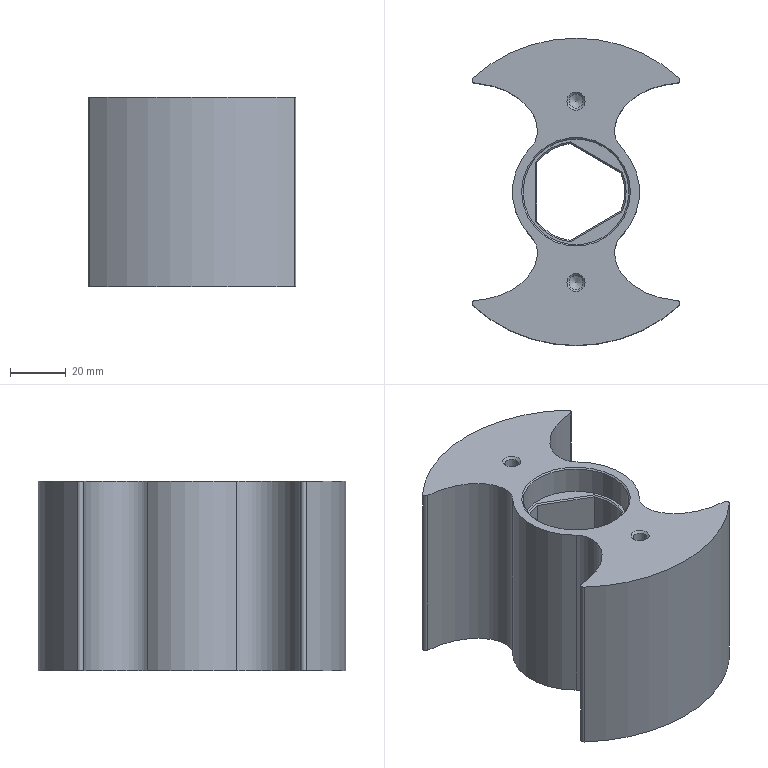NC program | NX | posted with a generic post | part box 74.46 x 110.159 x 68 mm
Lines 1 to 924 of 14265:
N10 G17 G21 G94 G90
(ZLEVEL_PROFILE_COPY_2 , TOOL : D25R0.5)
N12 T05 M6
N14 G54
N16 G17 G0 G90 X-62.643 Y50.68 S2000 M3
N18 G43 Z30. H5
N20 Z-0.349
N22 G94 G1 X-58.542 Y49.805 F1000.
N24 G3 X-56.163 Y50.576 R2.5
N26 G2 X-45.476 Y57.048 R21.659 F2200.
N28 X-34.718 Y57.049 R21.673
N30 G1 X-34.038 Y56.851
N32 G2 X-18.67 Y39.036 R21.585
N34 G1 X-18.667 Y39.034
N36 X-17.856 Y39.412
N38 X-17.06 Y39.763
N40 G2 X17.498 Y39.586 R43.327
N42 G1 X18.67 Y39.033
N44 G2 X19.13 Y41.403 R23.414
N46 G1 X19.344 Y42.145
N48 G2 X34.465 Y56.981 R21.564
N50 G1 X34.731 Y57.052
N52 G2 X45.481 Y57.045 R21.673
N54 X56.163 Y50.576 R21.656
N56 G3 X58.542 Y49.805 R2.5
N58 G1 X62.645 Y50.68
N60 G0 Z30.
N62 X-62.649 Y50.677
N64 Z-0.697
N66 G1 X-58.541 Y49.803 F1000.
N68 G3 X-56.163 Y50.576 R2.5
N70 G2 X-18.668 Y39.036 R21.625 F2200.
N72 X18.549 Y39.093 R43.271
N74 G1 X18.668 Y39.034
N76 G2 X56.163 Y50.576 R21.625
N78 G3 X58.541 Y49.803 R2.5
N80 G1 X62.649 Y50.677
N82 G0 Z30.
N84 X-62.649
N86 Z-1.046
N88 G1 X-58.541 Y49.803 F1000.
N90 G3 X-56.163 Y50.576 R2.5
N92 G2 X-18.668 Y39.036 R21.625 F2200.
N94 X18.549 Y39.093 R43.271
N96 G1 X18.668 Y39.034
N98 G2 X56.163 Y50.576 R21.625
N100 G3 X58.541 Y49.803 R2.5
N102 G1 X62.649 Y50.677
N104 G0 Z30.
N106 X-62.649
N108 Z-1.395
N110 G1 X-58.541 Y49.803 F1000.
N112 G3 X-56.163 Y50.576 R2.5
N114 G2 X-18.668 Y39.036 R21.625 F2200.
N116 X18.549 Y39.093 R43.271
N118 G1 X18.668 Y39.034
N120 G2 X56.163 Y50.576 R21.625
N122 G3 X58.541 Y49.803 R2.5
N124 G1 X62.649 Y50.677
N126 G0 Z30.
N128 X-62.649
N130 Z-1.744
N132 G1 X-58.541 Y49.803 F1000.
N134 G3 X-56.163 Y50.576 R2.5
N136 G2 X-18.668 Y39.036 R21.625 F2200.
N138 X18.549 Y39.093 R43.271
N140 G1 X18.668 Y39.034
N142 G2 X56.163 Y50.576 R21.625
N144 G3 X58.541 Y49.803 R2.5
N146 G1 X62.649 Y50.677
N148 G0 Z30.
N150 X-62.649
N152 Z-2.092
N154 G1 X-58.541 Y49.803 F1000.
N156 G3 X-56.163 Y50.576 R2.5
N158 G2 X-18.668 Y39.036 R21.625 F2200.
N160 X18.549 Y39.093 R43.271
N162 G1 X18.668 Y39.034
N164 G2 X56.163 Y50.576 R21.625
N166 G3 X58.541 Y49.803 R2.5
N168 G1 X62.649 Y50.677
N170 G0 Z30.
N172 X-62.649
N174 Z-2.441
N176 G1 X-58.541 Y49.803 F1000.
N178 G3 X-56.163 Y50.576 R2.5
N180 G2 X-18.668 Y39.036 R21.625 F2200.
N182 X18.549 Y39.093 R43.271
N184 G1 X18.668 Y39.034
N186 G2 X56.163 Y50.576 R21.625
N188 G3 X58.541 Y49.803 R2.5
N190 G1 X62.649 Y50.677
N192 G0 Z30.
N194 X-62.649
N196 Z-2.79
N198 G1 X-58.541 Y49.803 F1000.
N200 G3 X-56.163 Y50.576 R2.5
N202 G2 X-18.668 Y39.036 R21.625 F2200.
N204 X18.549 Y39.093 R43.271
N206 G1 X18.668 Y39.034
N208 G2 X56.163 Y50.576 R21.625
N210 G3 X58.541 Y49.803 R2.5
N212 G1 X62.649 Y50.677
N214 G0 Z30.
N216 X-62.649
N218 Z-3.138
N220 G1 X-58.541 Y49.803 F1000.
N222 G3 X-56.163 Y50.576 R2.5
N224 G2 X-18.668 Y39.036 R21.625 F2200.
N226 X18.549 Y39.093 R43.271
N228 G1 X18.668 Y39.034
N230 G2 X56.163 Y50.576 R21.625
N232 G3 X58.541 Y49.803 R2.5
N234 G1 X62.649 Y50.677
N236 G0 Z30.
N238 X-62.649
N240 Z-3.487
N242 G1 X-58.541 Y49.803 F1000.
N244 G3 X-56.163 Y50.576 R2.5
N246 G2 X-18.668 Y39.036 R21.625 F2200.
N248 X18.549 Y39.093 R43.271
N250 G1 X18.668 Y39.034
N252 G2 X56.163 Y50.576 R21.625
N254 G3 X58.541 Y49.803 R2.5
N256 G1 X62.649 Y50.677
N258 G0 Z30.
N260 X-62.649
N262 Z-3.836
N264 G1 X-58.541 Y49.803 F1000.
N266 G3 X-56.163 Y50.576 R2.5
N268 G2 X-18.668 Y39.036 R21.625 F2200.
N270 X18.549 Y39.093 R43.271
N272 G1 X18.668 Y39.034
N274 G2 X56.163 Y50.576 R21.625
N276 G3 X58.541 Y49.803 R2.5
N278 G1 X62.649 Y50.677
N280 G0 Z30.
N282 X-62.649
N284 Z-4.185
N286 G1 X-58.541 Y49.803 F1000.
N288 G3 X-56.163 Y50.576 R2.5
N290 G2 X-18.668 Y39.036 R21.625 F2200.
N292 X18.549 Y39.093 R43.271
N294 G1 X18.668 Y39.034
N296 G2 X56.163 Y50.576 R21.625
N298 G3 X58.541 Y49.803 R2.5
N300 G1 X62.649 Y50.677
N302 G0 Z30.
N304 X-62.649
N306 Z-4.533
N308 G1 X-58.541 Y49.803 F1000.
N310 G3 X-56.163 Y50.576 R2.5
N312 G2 X-18.668 Y39.036 R21.625 F2200.
N314 X18.549 Y39.093 R43.271
N316 G1 X18.668 Y39.034
N318 G2 X56.163 Y50.576 R21.625
N320 G3 X58.541 Y49.803 R2.5
N322 G1 X62.649 Y50.677
N324 G0 Z30.
N326 X-62.649
N328 Z-4.882
N330 G1 X-58.541 Y49.803 F1000.
N332 G3 X-56.163 Y50.576 R2.5
N334 G2 X-18.668 Y39.036 R21.625 F2200.
N336 X18.549 Y39.093 R43.271
N338 G1 X18.668 Y39.034
N340 G2 X56.163 Y50.576 R21.625
N342 G3 X58.541 Y49.803 R2.5
N344 G1 X62.649 Y50.677
N346 G0 Z30.
N348 X-62.649
N350 Z-5.231
N352 G1 X-58.541 Y49.803 F1000.
N354 G3 X-56.163 Y50.576 R2.5
N356 G2 X-18.668 Y39.036 R21.625 F2200.
N358 X18.549 Y39.093 R43.271
N360 G1 X18.668 Y39.034
N362 G2 X56.163 Y50.576 R21.625
N364 G3 X58.541 Y49.803 R2.5
N366 G1 X62.649 Y50.677
N368 G0 Z30.
N370 X-62.649
N372 Z-5.579
N374 G1 X-58.541 Y49.803 F1000.
N376 G3 X-56.163 Y50.576 R2.5
N378 G2 X-18.668 Y39.036 R21.625 F2200.
N380 X18.549 Y39.093 R43.271
N382 G1 X18.668 Y39.034
N384 G2 X56.163 Y50.576 R21.625
N386 G3 X58.541 Y49.803 R2.5
N388 G1 X62.649 Y50.677
N390 G0 Z30.
N392 X-62.649
N394 Z-5.928
N396 G1 X-58.541 Y49.803 F1000.
N398 G3 X-56.163 Y50.576 R2.5
N400 G2 X-18.668 Y39.036 R21.625 F2200.
N402 X18.549 Y39.093 R43.271
N404 G1 X18.668 Y39.035
N406 G2 X56.163 Y50.576 R21.625
N408 G3 X58.541 Y49.803 R2.5
N410 G1 X62.649 Y50.677
N412 G0 Z30.
N414 X-62.649
N416 Z-6.277
N418 G1 X-58.541 Y49.803 F1000.
N420 G3 X-56.163 Y50.576 R2.5
N422 G2 X-18.668 Y39.036 R21.625 F2200.
N424 X18.549 Y39.093 R43.271
N426 G1 X18.668 Y39.035
N428 G2 X56.163 Y50.576 R21.625
N430 G3 X58.541 Y49.803 R2.5
N432 G1 X62.649 Y50.677
N434 G0 Z30.
N436 X-62.649
N438 Z-6.626
N440 G1 X-58.541 Y49.803 F1000.
N442 G3 X-56.163 Y50.576 R2.5
N444 G2 X-18.668 Y39.036 R21.625 F2200.
N446 X18.549 Y39.093 R43.271
N448 G1 X18.668 Y39.035
N450 G2 X56.163 Y50.576 R21.625
N452 G3 X58.541 Y49.803 R2.5
N454 G1 X62.649 Y50.677
N456 G0 Z30.
N458 X-62.649
N460 Z-6.974
N462 G1 X-58.541 Y49.803 F1000.
N464 G3 X-56.163 Y50.576 R2.5
N466 G2 X-18.668 Y39.036 R21.625 F2200.
N468 X18.549 Y39.093 R43.271
N470 G1 X18.668 Y39.035
N472 G2 X56.163 Y50.576 R21.625
N474 G3 X58.541 Y49.803 R2.5
N476 G1 X62.649 Y50.677
N478 G0 Z30.
N480 X-62.649
N482 Z-7.323
N484 G1 X-58.541 Y49.803 F1000.
N486 G3 X-56.163 Y50.576 R2.5
N488 G2 X-18.668 Y39.036 R21.625 F2200.
N490 X18.549 Y39.093 R43.271
N492 G1 X18.668 Y39.035
N494 G2 X56.163 Y50.576 R21.625
N496 G3 X58.541 Y49.803 R2.5
N498 G1 X62.649 Y50.677
N500 G0 Z30.
N502 X-62.649
N504 Z-7.672
N506 G1 X-58.541 Y49.803 F1000.
N508 G3 X-56.163 Y50.576 R2.5
N510 G2 X-18.668 Y39.036 R21.625 F2200.
N512 X18.549 Y39.093 R43.271
N514 G1 X18.668 Y39.035
N516 G2 X56.163 Y50.576 R21.625
N518 G3 X58.541 Y49.803 R2.5
N520 G1 X62.649 Y50.677
N522 G0 Z30.
N524 X-62.649
N526 Z-8.021
N528 G1 X-58.541 Y49.803 F1000.
N530 G3 X-56.163 Y50.576 R2.5
N532 G2 X-18.668 Y39.036 R21.625 F2200.
N534 X18.549 Y39.093 R43.271
N536 G1 X18.668 Y39.035
N538 G2 X56.163 Y50.576 R21.625
N540 G3 X58.541 Y49.803 R2.5
N542 G1 X62.649 Y50.677
N544 G0 Z30.
N546 X-62.649
N548 Z-8.369
N550 G1 X-58.541 Y49.803 F1000.
N552 G3 X-56.163 Y50.576 R2.5
N554 G2 X-18.668 Y39.036 R21.625 F2200.
N556 X18.549 Y39.093 R43.271
N558 G1 X18.668 Y39.035
N560 G2 X56.163 Y50.576 R21.625
N562 G3 X58.541 Y49.803 R2.5
N564 G1 X62.649 Y50.677
N566 G0 Z30.
N568 X-62.649
N570 Z-8.718
N572 G1 X-58.541 Y49.803 F1000.
N574 G3 X-56.163 Y50.576 R2.5
N576 G2 X-18.668 Y39.036 R21.625 F2200.
N578 X18.549 Y39.093 R43.271
N580 G1 X18.668 Y39.035
N582 G2 X56.163 Y50.576 R21.625
N584 G3 X58.541 Y49.803 R2.5
N586 G1 X62.649 Y50.677
N588 G0 Z30.
N590 X-62.649
N592 Z-9.067
N594 G1 X-58.541 Y49.803 F1000.
N596 G3 X-56.163 Y50.576 R2.5
N598 G2 X-18.668 Y39.036 R21.625 F2200.
N600 X18.549 Y39.093 R43.271
N602 G1 X18.668 Y39.035
N604 G2 X56.163 Y50.576 R21.625
N606 G3 X58.541 Y49.803 R2.5
N608 G1 X62.649 Y50.677
N610 G0 Z30.
N612 X-62.649
N614 Z-9.415
N616 G1 X-58.541 Y49.803 F1000.
N618 G3 X-56.163 Y50.576 R2.5
N620 G2 X-18.668 Y39.036 R21.625 F2200.
N622 X18.549 Y39.093 R43.271
N624 G1 X18.668 Y39.035
N626 G2 X56.163 Y50.576 R21.625
N628 G3 X58.541 Y49.803 R2.5
N630 G1 X62.649 Y50.677
N632 G0 Z30.
N634 X-62.649
N636 Z-9.764
N638 G1 X-58.541 Y49.803 F1000.
N640 G3 X-56.163 Y50.576 R2.5
N642 G2 X-18.668 Y39.036 R21.625 F2200.
N644 X18.549 Y39.093 R43.271
N646 G1 X18.668 Y39.035
N648 G2 X56.163 Y50.576 R21.625
N650 G3 X58.541 Y49.803 R2.5
N652 G1 X62.649 Y50.677
N654 G0 Z30.
N656 X-62.649
N658 Z-10.113
N660 G1 X-58.541 Y49.803 F1000.
N662 G3 X-56.163 Y50.576 R2.5
N664 G2 X-18.668 Y39.036 R21.625 F2200.
N666 X18.549 Y39.093 R43.271
N668 G1 X18.668 Y39.035
N670 G2 X56.163 Y50.576 R21.625
N672 G3 X58.541 Y49.803 R2.5
N674 G1 X62.649 Y50.677
N676 G0 Z30.
N678 X-62.649
N680 Z-10.462
N682 G1 X-58.541 Y49.803 F1000.
N684 G3 X-56.163 Y50.576 R2.5
N686 G2 X-18.668 Y39.036 R21.625 F2200.
N688 X18.549 Y39.093 R43.271
N690 G1 X18.668 Y39.035
N692 G2 X56.163 Y50.576 R21.625
N694 G3 X58.541 Y49.803 R2.5
N696 G1 X62.649 Y50.677
N698 G0 Z30.
N700 X-62.649
N702 Z-10.81
N704 G1 X-58.541 Y49.803 F1000.
N706 G3 X-56.163 Y50.576 R2.5
N708 G2 X-18.668 Y39.036 R21.625 F2200.
N710 X18.549 Y39.093 R43.271
N712 G1 X18.668 Y39.035
N714 G2 X56.163 Y50.576 R21.625
N716 G3 X58.541 Y49.803 R2.5
N718 G1 X62.649 Y50.677
N720 G0 Z30.
N722 X-62.649
N724 Z-11.159
N726 G1 X-58.541 Y49.803 F1000.
N728 G3 X-56.163 Y50.576 R2.5
N730 G2 X-18.668 Y39.036 R21.625 F2200.
N732 X18.549 Y39.093 R43.271
N734 G1 X18.668 Y39.035
N736 G2 X56.163 Y50.576 R21.625
N738 G3 X58.541 Y49.803 R2.5
N740 G1 X62.649 Y50.677
N742 G0 Z30.
N744 X-62.649
N746 Z-11.508
N748 G1 X-58.541 Y49.803 F1000.
N750 G3 X-56.163 Y50.576 R2.5
N752 G2 X-18.668 Y39.036 R21.625 F2200.
N754 X18.549 Y39.093 R43.271
N756 G1 X18.668 Y39.035
N758 G2 X56.163 Y50.576 R21.625
N760 G3 X58.541 Y49.803 R2.5
N762 G1 X62.649 Y50.677
N764 G0 Z30.
N766 X-62.649
N768 Z-11.856
N770 G1 X-58.541 Y49.803 F1000.
N772 G3 X-56.163 Y50.576 R2.5
N774 G2 X-18.668 Y39.036 R21.625 F2200.
N776 X18.549 Y39.093 R43.271
N778 G1 X18.668 Y39.035
N780 G2 X56.163 Y50.576 R21.625
N782 G3 X58.541 Y49.803 R2.5
N784 G1 X62.649 Y50.677
N786 G0 Z30.
N788 X-62.649
N790 Z-12.205
N792 G1 X-58.541 Y49.803 F1000.
N794 G3 X-56.163 Y50.576 R2.5
N796 G2 X-18.668 Y39.036 R21.625 F2200.
N798 X18.549 Y39.093 R43.271
N800 G1 X18.668 Y39.035
N802 G2 X56.163 Y50.576 R21.625
N804 G3 X58.541 Y49.803 R2.5
N806 G1 X62.649 Y50.677
N808 G0 Z30.
N810 X-62.649
N812 Z-12.554
N814 G1 X-58.541 Y49.803 F1000.
N816 G3 X-56.163 Y50.576 R2.5
N818 G2 X-18.668 Y39.036 R21.625 F2200.
N820 X18.549 Y39.093 R43.271
N822 G1 X18.668 Y39.035
N824 G2 X56.163 Y50.576 R21.625
N826 G3 X58.541 Y49.803 R2.5
N828 G1 X62.649 Y50.677
N830 G0 Z30.
N832 X-62.649
N834 Z-12.903
N836 G1 X-58.541 Y49.803 F1000.
N838 G3 X-56.163 Y50.576 R2.5
N840 G2 X-18.668 Y39.036 R21.625 F2200.
N842 X18.549 Y39.093 R43.271
N844 G1 X18.668 Y39.035
N846 G2 X56.163 Y50.576 R21.625
N848 G3 X58.541 Y49.803 R2.5
N850 G1 X62.649 Y50.677
N852 G0 Z30.
N854 X-62.649
N856 Z-13.251
N858 G1 X-58.541 Y49.803 F1000.
N860 G3 X-56.163 Y50.576 R2.5
N862 G2 X-18.668 Y39.036 R21.625 F2200.
N864 X18.549 Y39.093 R43.271
N866 G1 X18.668 Y39.035
N868 G2 X56.163 Y50.576 R21.625
N870 G3 X58.541 Y49.803 R2.5
N872 G1 X62.649 Y50.677
N874 G0 Z30.
N876 X-62.649
N878 Z-13.6
N880 G1 X-58.541 Y49.803 F1000.
N882 G3 X-56.163 Y50.576 R2.5
N884 G2 X-18.668 Y39.036 R21.625 F2200.
N886 X18.549 Y39.093 R43.271
N888 G1 X18.668 Y39.035
N890 G2 X56.163 Y50.576 R21.625
N892 G3 X58.541 Y49.803 R2.5
N894 G1 X62.649 Y50.677
N896 G0 Z30.
N898 X-62.649
N900 Z-13.949
N902 G1 X-58.541 Y49.803 F1000.
N904 G3 X-56.163 Y50.576 R2.5
N906 G2 X-18.668 Y39.036 R21.625 F2200.
N908 X18.549 Y39.093 R43.271
N910 G1 X18.668 Y39.035
N912 G2 X56.163 Y50.576 R21.625
N914 G3 X58.541 Y49.803 R2.5
N916 G1 X62.649 Y50.677
N918 G0 Z30.
N920 X-62.649
N922 Z-14.297
N924 G1 X-58.541 Y49.803 F1000.
N926 G3 X-56.163 Y50.576 R2.5
N928 G2 X-18.668 Y39.036 R21.625 F2200.
N930 X18.549 Y39.093 R43.271
N932 G1 X18.668 Y39.035
N934 G2 X56.163 Y50.576 R21.625
N936 G3 X58.541 Y49.803 R2.5
N938 G1 X62.649 Y50.677
N940 G0 Z30.
N942 X-62.649
N944 Z-14.646
N946 G1 X-58.541 Y49.803 F1000.
N948 G3 X-56.163 Y50.576 R2.5
N950 G2 X-18.668 Y39.036 R21.625 F2200.
N952 X18.549 Y39.093 R43.271
N954 G1 X18.668 Y39.035
N956 G2 X56.163 Y50.576 R21.625
N958 G3 X58.541 Y49.803 R2.5
N960 G1 X62.649 Y50.677
N962 G0 Z30.
N964 X-62.649
N966 Z-14.995
N968 G1 X-58.541 Y49.803 F1000.
N970 G3 X-56.163 Y50.576 R2.5
N972 G2 X-18.668 Y39.036 R21.625 F2200.
N974 X18.549 Y39.093 R43.271
N976 G1 X18.668 Y39.035
N978 G2 X56.163 Y50.576 R21.625
N980 G3 X58.541 Y49.803 R2.5
N982 G1 X62.649 Y50.677
N984 G0 Z30.
N986 X-62.649
N988 Z-15.344
N990 G1 X-58.541 Y49.803 F1000.
N992 G3 X-56.163 Y50.576 R2.5
N994 G2 X-18.668 Y39.036 R21.625 F2200.
N996 X18.549 Y39.093 R43.271
N998 G1 X18.668 Y39.035
N1000 G2 X56.163 Y50.576 R21.625
N1002 G3 X58.541 Y49.803 R2.5
N1004 G1 X62.649 Y50.677
N1006 G0 Z30.
N1008 X-62.649
N1010 Z-15.692
N1012 G1 X-58.541 Y49.803 F1000.
N1014 G3 X-56.163 Y50.576 R2.5
N1016 G2 X-18.668 Y39.036 R21.625 F2200.
N1018 X18.549 Y39.093 R43.271
N1020 G1 X18.668 Y39.035
N1022 G2 X56.163 Y50.576 R21.625
N1024 G3 X58.541 Y49.803 R2.5
N1026 G1 X62.649 Y50.677
N1028 G0 Z30.
N1030 X-62.649
N1032 Z-16.041
N1034 G1 X-58.541 Y49.803 F1000.
N1036 G3 X-56.163 Y50.576 R2.5
N1038 G2 X-18.668 Y39.036 R21.625 F2200.
N1040 X18.549 Y39.093 R43.271
N1042 G1 X18.668 Y39.035
N1044 G2 X56.163 Y50.576 R21.625
N1046 G3 X58.541 Y49.803 R2.5
N1048 G1 X62.649 Y50.677
N1050 G0 Z30.
N1052 X-62.649
N1054 Z-16.39
N1056 G1 X-58.541 Y49.803 F1000.
N1058 G3 X-56.163 Y50.576 R2.5
N1060 G2 X-18.668 Y39.036 R21.625 F2200.
N1062 X18.549 Y39.093 R43.271
N1064 G1 X18.668 Y39.035
N1066 G2 X56.163 Y50.576 R21.625
N1068 G3 X58.541 Y49.803 R2.5
N1070 G1 X62.649 Y50.677
N1072 G0 Z30.
N1074 X-62.649
N1076 Z-16.738
N1078 G1 X-58.541 Y49.803 F1000.
N1080 G3 X-56.163 Y50.576 R2.5
N1082 G2 X-18.668 Y39.036 R21.625 F2200.
N1084 X18.549 Y39.093 R43.271
N1086 G1 X18.668 Y39.035
N1088 G2 X56.163 Y50.576 R21.625
N1090 G3 X58.541 Y49.803 R2.5
N1092 G1 X62.649 Y50.677
N1094 G0 Z30.
N1096 X-62.649
N1098 Z-17.087
N1100 G1 X-58.541 Y49.803 F1000.
N1102 G3 X-56.163 Y50.576 R2.5
N1104 G2 X-18.668 Y39.036 R21.625 F2200.
N1106 X18.549 Y39.093 R43.271
N1108 G1 X18.668 Y39.035
N1110 G2 X56.163 Y50.576 R21.625
N1112 G3 X58.541 Y49.803 R2.5
N1114 G1 X62.649 Y50.677
N1116 G0 Z30.
N1118 X-62.649
N1120 Z-17.436
N1122 G1 X-58.541 Y49.803 F1000.
N1124 G3 X-56.163 Y50.576 R2.5
N1126 G2 X-18.668 Y39.036 R21.625 F2200.
N1128 X18.549 Y39.093 R43.271
N1130 G1 X18.668 Y39.035
N1132 G2 X56.163 Y50.576 R21.625
N1134 G3 X58.541 Y49.803 R2.5
N1136 G1 X62.649 Y50.677
N1138 G0 Z30.
N1140 X-62.649
N1142 Z-17.785
N1144 G1 X-58.541 Y49.803 F1000.
N1146 G3 X-56.163 Y50.576 R2.5
N1148 G2 X-18.668 Y39.036 R21.625 F2200.
N1150 X18.549 Y39.093 R43.271
N1152 G1 X18.668 Y39.035
N1154 G2 X56.163 Y50.576 R21.625
N1156 G3 X58.541 Y49.803 R2.5
N1158 G1 X62.649 Y50.677
N1160 G0 Z30.
N1162 X-62.649
N1164 Z-18.133
N1166 G1 X-58.541 Y49.803 F1000.
N1168 G3 X-56.163 Y50.576 R2.5
N1170 G2 X-18.668 Y39.036 R21.625 F2200.
N1172 X18.549 Y39.093 R43.271
N1174 G1 X18.668 Y39.035
N1176 G2 X56.163 Y50.576 R21.625
N1178 G3 X58.541 Y49.803 R2.5
N1180 G1 X62.649 Y50.677
N1182 G0 Z30.
N1184 X-62.649
N1186 Z-18.482
N1188 G1 X-58.541 Y49.803 F1000.
N1190 G3 X-56.163 Y50.576 R2.5
N1192 G2 X-18.668 Y39.036 R21.625 F2200.
N1194 X18.549 Y39.093 R43.271
N1196 G1 X18.668 Y39.035
N1198 G2 X56.163 Y50.576 R21.625
N1200 G3 X58.541 Y49.803 R2.5
N1202 G1 X62.649 Y50.677
N1204 G0 Z30.
N1206 X-62.649
N1208 Z-18.831
N1210 G1 X-58.541 Y49.803 F1000.
N1212 G3 X-56.163 Y50.576 R2.5
N1214 G2 X-18.668 Y39.036 R21.625 F2200.
N1216 X18.549 Y39.093 R43.271
N1218 G1 X18.668 Y39.035
N1220 G2 X56.163 Y50.576 R21.625
N1222 G3 X58.541 Y49.803 R2.5
N1224 G1 X62.649 Y50.677
N1226 G0 Z30.
N1228 X-62.649
N1230 Z-19.179
N1232 G1 X-58.541 Y49.803 F1000.
N1234 G3 X-56.163 Y50.576 R2.5
N1236 G2 X-18.668 Y39.036 R21.625 F2200.
N1238 X18.549 Y39.093 R43.271
N1240 G1 X18.668 Y39.035
N1242 G2 X56.163 Y50.576 R21.625
N1244 G3 X58.541 Y49.803 R2.5
N1246 G1 X62.649 Y50.677
N1248 G0 Z30.
N1250 X-62.649
N1252 Z-19.528
N1254 G1 X-58.541 Y49.803 F1000.
N1256 G3 X-56.163 Y50.576 R2.5
N1258 G2 X-18.668 Y39.036 R21.625 F2200.
N1260 X18.549 Y39.093 R43.271
N1262 G1 X18.668 Y39.035
N1264 G2 X56.163 Y50.576 R21.625
N1266 G3 X58.541 Y49.803 R2.5
N1268 G1 X62.649 Y50.677
N1270 G0 Z30.
N1272 X-62.649
N1274 Z-19.877
N1276 G1 X-58.541 Y49.803 F1000.
N1278 G3 X-56.163 Y50.576 R2.5
N1280 G2 X-18.668 Y39.036 R21.625 F2200.
N1282 X18.549 Y39.093 R43.271
N1284 G1 X18.668 Y39.035
N1286 G2 X56.163 Y50.576 R21.625
N1288 G3 X58.541 Y49.803 R2.5
N1290 G1 X62.649 Y50.677
N1292 G0 Z30.
N1294 X-62.649
N1296 Z-20.226
N1298 G1 X-58.541 Y49.803 F1000.
N1300 G3 X-56.163 Y50.576 R2.5
N1302 G2 X-18.668 Y39.036 R21.625 F2200.
N1304 X18.549 Y39.093 R43.271
N1306 G1 X18.668 Y39.035
N1308 G2 X56.163 Y50.576 R21.625
N1310 G3 X58.541 Y49.803 R2.5
N1312 G1 X62.649 Y50.677
N1314 G0 Z30.
N1316 X-62.649
N1318 Z-20.574
N1320 G1 X-58.541 Y49.803 F1000.
N1322 G3 X-56.163 Y50.576 R2.5
N1324 G2 X-18.668 Y39.036 R21.625 F2200.
N1326 X18.549 Y39.093 R43.271
N1328 G1 X18.668 Y39.035
N1330 G2 X56.163 Y50.576 R21.625
N1332 G3 X58.541 Y49.803 R2.5
N1334 G1 X62.649 Y50.677
N1336 G0 Z30.
N1338 X-62.649
N1340 Z-20.923
N1342 G1 X-58.541 Y49.803 F1000.
N1344 G3 X-56.163 Y50.576 R2.5
N1346 G2 X-18.668 Y39.036 R21.625 F2200.
N1348 X18.549 Y39.093 R43.271
N1350 G1 X18.668 Y39.035
N1352 G2 X56.163 Y50.576 R21.625
N1354 G3 X58.541 Y49.803 R2.5
N1356 G1 X62.649 Y50.677
N1358 G0 Z30.
N1360 X-62.649
N1362 Z-21.272
N1364 G1 X-58.541 Y49.803 F1000.
N1366 G3 X-56.163 Y50.576 R2.5
N1368 G2 X-18.668 Y39.036 R21.625 F2200.
N1370 X18.549 Y39.093 R43.271
N1372 G1 X18.668 Y39.035
N1374 G2 X56.163 Y50.576 R21.625
N1376 G3 X58.541 Y49.803 R2.5
N1378 G1 X62.649 Y50.677
N1380 G0 Z30.
N1382 X-62.649
N1384 Z-21.621
N1386 G1 X-58.541 Y49.803 F1000.
N1388 G3 X-56.163 Y50.576 R2.5
N1390 G2 X-18.668 Y39.036 R21.625 F2200.
N1392 X18.549 Y39.093 R43.271
N1394 G1 X18.668 Y39.035
N1396 G2 X56.163 Y50.576 R21.625
N1398 G3 X58.541 Y49.803 R2.5
N1400 G1 X62.649 Y50.677
N1402 G0 Z30.
N1404 X-62.649
N1406 Z-21.969
N1408 G1 X-58.541 Y49.803 F1000.
N1410 G3 X-56.163 Y50.576 R2.5
N1412 G2 X-18.668 Y39.036 R21.625 F2200.
N1414 X18.549 Y39.093 R43.271
N1416 G1 X18.668 Y39.035
N1418 G2 X56.163 Y50.576 R21.625
N1420 G3 X58.541 Y49.803 R2.5
N1422 G1 X62.649 Y50.677
N1424 G0 Z30.
N1426 X-62.649
N1428 Z-22.318
N1430 G1 X-58.541 Y49.803 F1000.
N1432 G3 X-56.163 Y50.576 R2.5
N1434 G2 X-18.668 Y39.036 R21.625 F2200.
N1436 X18.549 Y39.093 R43.271
N1438 G1 X18.668 Y39.035
N1440 G2 X56.163 Y50.576 R21.625
N1442 G3 X58.541 Y49.803 R2.5
N1444 G1 X62.649 Y50.677
N1446 G0 Z30.
N1448 X-62.649
N1450 Z-22.667
N1452 G1 X-58.541 Y49.803 F1000.
N1454 G3 X-56.163 Y50.576 R2.5
N1456 G2 X-18.668 Y39.036 R21.625 F2200.
N1458 X18.549 Y39.093 R43.271
N1460 G1 X18.668 Y39.035
N1462 G2 X56.163 Y50.576 R21.625
N1464 G3 X58.541 Y49.803 R2.5
N1466 G1 X62.649 Y50.677
N1468 G0 Z30.
N1470 X-62.649
N1472 Z-23.015
N1474 G1 X-58.541 Y49.803 F1000.
N1476 G3 X-56.163 Y50.576 R2.5
N1478 G2 X-18.668 Y39.036 R21.625 F2200.
N1480 X18.549 Y39.093 R43.271
N1482 G1 X18.668 Y39.035
N1484 G2 X56.163 Y50.576 R21.625
N1486 G3 X58.541 Y49.803 R2.5
N1488 G1 X62.649 Y50.677
N1490 G0 Z30.
N1492 X-62.649
N1494 Z-23.364
N1496 G1 X-58.541 Y49.803 F1000.
N1498 G3 X-56.163 Y50.576 R2.5
N1500 G2 X-18.668 Y39.036 R21.625 F2200.
N1502 X18.549 Y39.093 R43.271
N1504 G1 X18.668 Y39.035
N1506 G2 X56.163 Y50.576 R21.625
N1508 G3 X58.541 Y49.803 R2.5
N1510 G1 X62.649 Y50.677
N1512 G0 Z30.
N1514 X-62.649
N1516 Z-23.713
N1518 G1 X-58.541 Y49.803 F1000.
N1520 G3 X-56.163 Y50.576 R2.5
N1522 G2 X-18.668 Y39.036 R21.625 F2200.
N1524 X18.549 Y39.093 R43.271
N1526 G1 X18.668 Y39.035
N1528 G2 X56.163 Y50.576 R21.625
N1530 G3 X58.541 Y49.803 R2.5
N1532 G1 X62.649 Y50.677
N1534 G0 Z30.
N1536 X-62.649
N1538 Z-24.062
N1540 G1 X-58.541 Y49.803 F1000.
N1542 G3 X-56.163 Y50.576 R2.5
N1544 G2 X-18.668 Y39.036 R21.625 F2200.
N1546 X18.549 Y39.093 R43.271
N1548 G1 X18.668 Y39.035
N1550 G2 X56.163 Y50.576 R21.625
N1552 G3 X58.541 Y49.803 R2.5
N1554 G1 X62.649 Y50.677
N1556 G0 Z30.
N1558 X-62.649
N1560 Z-24.41
N1562 G1 X-58.541 Y49.803 F1000.
N1564 G3 X-56.163 Y50.576 R2.5
N1566 G2 X-18.668 Y39.036 R21.625 F2200.
N1568 X18.549 Y39.093 R43.271
N1570 G1 X18.668 Y39.035
N1572 G2 X56.163 Y50.576 R21.625
N1574 G3 X58.541 Y49.803 R2.5
N1576 G1 X62.649 Y50.677
N1578 G0 Z30.
N1580 X-62.649
N1582 Z-24.759
N1584 G1 X-58.541 Y49.803 F1000.
N1586 G3 X-56.163 Y50.576 R2.5
N1588 G2 X-18.668 Y39.036 R21.625 F2200.
N1590 X18.549 Y39.093 R43.271
N1592 G1 X18.668 Y39.035
N1594 G2 X56.163 Y50.576 R21.625
N1596 G3 X58.541 Y49.803 R2.5
N1598 G1 X62.649 Y50.677
N1600 G0 Z30.
N1602 X-62.649
N1604 Z-25.108
N1606 G1 X-58.541 Y49.803 F1000.
N1608 G3 X-56.163 Y50.576 R2.5
N1610 G2 X-18.668 Y39.036 R21.625 F2200.
N1612 X18.549 Y39.093 R43.271
N1614 G1 X18.668 Y39.035
N1616 G2 X56.163 Y50.576 R21.625
N1618 G3 X58.541 Y49.803 R2.5
N1620 G1 X62.649 Y50.677
N1622 G0 Z30.
N1624 X-62.649
N1626 Z-25.456
N1628 G1 X-58.541 Y49.803 F1000.
N1630 G3 X-56.163 Y50.576 R2.5
N1632 G2 X-18.668 Y39.036 R21.625 F2200.
N1634 X18.549 Y39.093 R43.271
N1636 G1 X18.668 Y39.035
N1638 G2 X56.163 Y50.576 R21.625
N1640 G3 X58.541 Y49.803 R2.5
N1642 G1 X62.649 Y50.677
N1644 G0 Z30.
N1646 X-62.649
N1648 Z-25.805
N1650 G1 X-58.541 Y49.803 F1000.
N1652 G3 X-56.163 Y50.576 R2.5
N1654 G2 X-18.668 Y39.036 R21.625 F2200.
N1656 X18.549 Y39.093 R43.271
N1658 G1 X18.668 Y39.035
N1660 G2 X56.163 Y50.576 R21.625
N1662 G3 X58.541 Y49.803 R2.5
N1664 G1 X62.649 Y50.677
N1666 G0 Z30.
N1668 X-62.649
N1670 Z-26.154
N1672 G1 X-58.541 Y49.803 F1000.
N1674 G3 X-56.163 Y50.576 R2.5
N1676 G2 X-18.668 Y39.036 R21.625 F2200.
N1678 X18.549 Y39.093 R43.271
N1680 G1 X18.668 Y39.035
N1682 G2 X56.163 Y50.576 R21.625
N1684 G3 X58.541 Y49.803 R2.5
N1686 G1 X62.649 Y50.677
N1688 G0 Z30.
N1690 X-62.649
N1692 Z-26.503
N1694 G1 X-58.541 Y49.803 F1000.
N1696 G3 X-56.163 Y50.576 R2.5
N1698 G2 X-18.668 Y39.036 R21.625 F2200.
N1700 X18.549 Y39.093 R43.271
N1702 G1 X18.668 Y39.035
N1704 G2 X56.163 Y50.576 R21.625
N1706 G3 X58.541 Y49.803 R2.5
N1708 G1 X62.649 Y50.677
N1710 G0 Z30.
N1712 X-62.649
N1714 Z-26.851
N1716 G1 X-58.541 Y49.803 F1000.
N1718 G3 X-56.163 Y50.576 R2.5
N1720 G2 X-18.668 Y39.036 R21.625 F2200.
N1722 X18.549 Y39.093 R43.271
N1724 G1 X18.668 Y39.035
N1726 G2 X56.163 Y50.576 R21.625
N1728 G3 X58.541 Y49.803 R2.5
N1730 G1 X62.649 Y50.677
N1732 G0 Z30.
N1734 X-62.649
N1736 Z-27.2
N1738 G1 X-58.541 Y49.803 F1000.
N1740 G3 X-56.163 Y50.576 R2.5
N1742 G2 X-18.668 Y39.036 R21.625 F2200.
N1744 X18.549 Y39.093 R43.271
N1746 G1 X18.668 Y39.035
N1748 G2 X56.163 Y50.576 R21.625
N1750 G3 X58.541 Y49.803 R2.5
N1752 G1 X62.649 Y50.677
N1754 G0 Z30.
N1756 X-62.649
N1758 Z-27.549
N1760 G1 X-58.541 Y49.803 F1000.
N1762 G3 X-56.163 Y50.576 R2.5
N1764 G2 X-18.668 Y39.036 R21.625 F2200.
N1766 X18.549 Y39.093 R43.271
N1768 G1 X18.668 Y39.035
N1770 G2 X56.163 Y50.576 R21.625
N1772 G3 X58.541 Y49.803 R2.5
N1774 G1 X62.649 Y50.677
N1776 G0 Z30.
N1778 X-62.649
N1780 Z-27.897
N1782 G1 X-58.541 Y49.803 F1000.
N1784 G3 X-56.163 Y50.576 R2.5
N1786 G2 X-18.668 Y39.036 R21.625 F2200.
N1788 X18.549 Y39.093 R43.271
N1790 G1 X18.668 Y39.035
N1792 G2 X56.163 Y50.576 R21.625
N1794 G3 X58.541 Y49.803 R2.5
N1796 G1 X62.649 Y50.677
N1798 G0 Z30.
N1800 X-62.649
N1802 Z-28.246
N1804 G1 X-58.541 Y49.803 F1000.
N1806 G3 X-56.163 Y50.576 R2.5
N1808 G2 X-18.668 Y39.036 R21.625 F2200.
N1810 X18.549 Y39.093 R43.271
N1812 G1 X18.668 Y39.035
N1814 G2 X56.163 Y50.576 R21.625
N1816 G3 X58.541 Y49.803 R2.5
N1818 G1 X62.649 Y50.677
N1820 G0 Z30.
N1822 X-62.649
N1824 Z-28.595
N1826 G1 X-58.541 Y49.803 F1000.
N1828 G3 X-56.163 Y50.576 R2.5
N1830 G2 X-18.668 Y39.036 R21.625 F2200.
N1832 X18.549 Y39.093 R43.271
N1834 G1 X18.668 Y39.035
N1836 G2 X56.163 Y50.576 R21.625
N1838 G3 X58.541 Y49.803 R2.5
N1840 G1 X62.649 Y50.677
N1842 G0 Z30.
N1844 X-62.649
N1846 Z-28.944